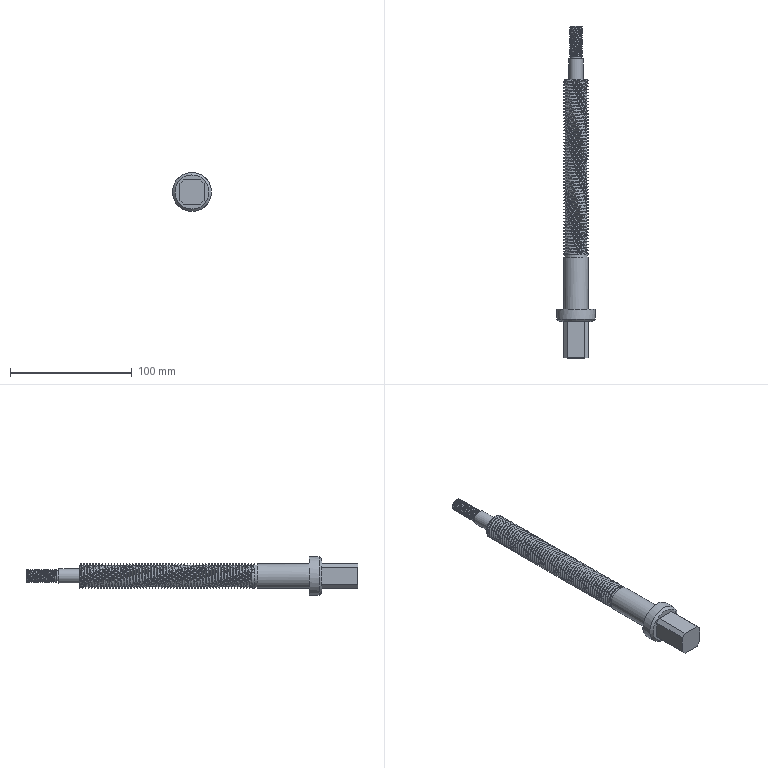Part | NX | features EXTRUDE 8, DATUM_CSYS 7, SKETCH 6, CHAMFER 2, THREADS 2 | 1 solid | 33 faces | box 32 x 273 x 32 mm | volume 74407 mm3 | plane 19 | cylinder 9 | spline 4 | cone 1 | commonest cylinder face diameters 20 x2 8.5 x1 9 x1 10 x1 12 x1 17.5 x1